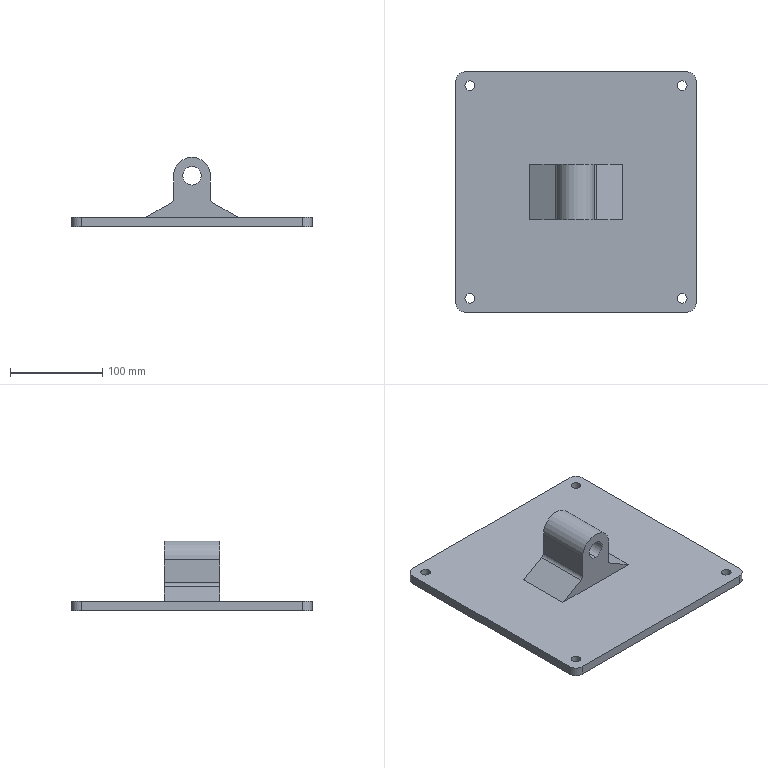Part | SolidWorks | features ICE 2, Extrusion 1, Fillet 1 | 1 solid | 29 faces | box 260 x 260 x 75 mm | volume 829791 mm3 | cylinder 17 | plane 12 | commonest cylinder face diameters 10.5 x8 20 x6 10 x2 40 x1
STEP:
#1=CARTESIAN_POINT('',(0.,30.,45.));
#2=VERTEX_POINT('',#1);
#3=CARTESIAN_POINT('',(0.,30.,65.));
#4=VERTEX_POINT('',#3);
#5=CARTESIAN_POINT('',(0.,30.,55.));
#6=DIRECTION('',(0.,1.,0.));
#7=DIRECTION('',(0.,0.,1.));
#8=AXIS2_PLACEMENT_3D('',#5,#6,#7);
#9=CIRCLE('',#8,10.);
#10=EDGE_CURVE('',#2,#4,#9,.T.);
#11=ORIENTED_EDGE('',*,*,#10,.T.);
#12=CARTESIAN_POINT('',(0.,-30.,65.));
#13=VERTEX_POINT('',#12);
#14=CARTESIAN_POINT('',(0.,104.,65.));
#15=DIRECTION('',(0.,-1.,0.));
#16=VECTOR('',#15,1000.);
#17=LINE('',#14,#16);
#18=EDGE_CURVE('',#4,#13,#17,.T.);
#19=ORIENTED_EDGE('',*,*,#18,.T.);
#20=CARTESIAN_POINT('',(0.,-30.,45.));
#21=VERTEX_POINT('',#20);
#22=CARTESIAN_POINT('',(0.,-30.,55.));
#23=DIRECTION('',(0.,-1.,0.));
#24=DIRECTION('',(0.,0.,-1.));
#25=AXIS2_PLACEMENT_3D('',#22,#23,#24);
#26=CIRCLE('',#25,10.);
#27=EDGE_CURVE('',#13,#21,#26,.T.);
#28=ORIENTED_EDGE('',*,*,#27,.T.);
#29=CARTESIAN_POINT('',(0.,104.,45.));
#30=DIRECTION('',(0.,-1.,0.));
#31=VECTOR('',#30,1000.);
#32=LINE('',#29,#31);
#33=EDGE_CURVE('',#2,#21,#32,.T.);
#34=ORIENTED_EDGE('',*,*,#33,.F.);
#35=EDGE_LOOP('',(#11,#19,#28,#34));
#36=FACE_OUTER_BOUND('',#35,.T.);
#37=CARTESIAN_POINT('',(0.,104.,55.));
#38=DIRECTION('',(0.,-1.,0.));
#39=DIRECTION('',(0.,0.,-1.));
#40=AXIS2_PLACEMENT_3D('',#37,#38,#39);
#41=CYLINDRICAL_SURFACE('',#40,10.);
#42=ADVANCED_FACE('',(#36),#41,.F.);
#43=CARTESIAN_POINT('',(-120.25,-115.,10.));
#44=VERTEX_POINT('',#43);
#45=CARTESIAN_POINT('',(-109.75,-115.,10.));
#46=VERTEX_POINT('',#45);
#47=CARTESIAN_POINT('',(-115.,-115.,10.));
#48=DIRECTION('',(0.,0.,1.));
#49=DIRECTION('',(1.,0.,0.));
#50=AXIS2_PLACEMENT_3D('',#47,#48,#49);
#51=CIRCLE('',#50,5.25);
#52=EDGE_CURVE('',#44,#46,#51,.T.);
#53=ORIENTED_EDGE('',*,*,#52,.T.);
#54=CARTESIAN_POINT('',(-109.75,-115.,0.));
#55=VERTEX_POINT('',#54);
#56=CARTESIAN_POINT('',(-109.75,-115.,10.));
#57=DIRECTION('',(0.,0.,-1.));
#58=VECTOR('',#57,1000.);
#59=LINE('',#56,#58);
#60=EDGE_CURVE('',#46,#55,#59,.T.);
#61=ORIENTED_EDGE('',*,*,#60,.T.);
#62=CARTESIAN_POINT('',(-120.25,-115.,0.));
#63=VERTEX_POINT('',#62);
#64=CARTESIAN_POINT('',(-115.,-115.,0.));
#65=DIRECTION('',(0.,0.,1.));
#66=DIRECTION('',(1.,0.,0.));
#67=AXIS2_PLACEMENT_3D('',#64,#65,#66);
#68=CIRCLE('',#67,5.25);
#69=EDGE_CURVE('',#63,#55,#68,.T.);
#70=ORIENTED_EDGE('',*,*,#69,.F.);
#71=CARTESIAN_POINT('',(-120.25,-115.,10.));
#72=DIRECTION('',(0.,0.,-1.));
#73=VECTOR('',#72,1000.);
#74=LINE('',#71,#73);
#75=EDGE_CURVE('',#44,#63,#74,.T.);
#76=ORIENTED_EDGE('',*,*,#75,.F.);
#77=EDGE_LOOP('',(#53,#61,#70,#76));
#78=FACE_OUTER_BOUND('',#77,.T.);
#79=CARTESIAN_POINT('',(-115.,-115.,10.));
#80=DIRECTION('',(0.,0.,-1.));
#81=DIRECTION('',(-1.,0.,0.));
#82=AXIS2_PLACEMENT_3D('',#79,#80,#81);
#83=CYLINDRICAL_SURFACE('',#82,5.25);
#84=ADVANCED_FACE('',(#78),#83,.F.);
#85=CARTESIAN_POINT('',(109.75,-115.,10.));
#86=VERTEX_POINT('',#85);
#87=CARTESIAN_POINT('',(120.25,-115.,10.));
#88=VERTEX_POINT('',#87);
#89=CARTESIAN_POINT('',(115.,-115.,10.));
#90=DIRECTION('',(0.,0.,1.));
#91=DIRECTION('',(1.,0.,0.));
#92=AXIS2_PLACEMENT_3D('',#89,#90,#91);
#93=CIRCLE('',#92,5.25);
#94=EDGE_CURVE('',#86,#88,#93,.T.);
#95=ORIENTED_EDGE('',*,*,#94,.T.);
#96=CARTESIAN_POINT('',(120.25,-115.,0.));
#97=VERTEX_POINT('',#96);
#98=CARTESIAN_POINT('',(120.25,-115.,10.));
#99=DIRECTION('',(0.,0.,-1.));
#100=VECTOR('',#99,1000.);
#101=LINE('',#98,#100);
#102=EDGE_CURVE('',#88,#97,#101,.T.);
#103=ORIENTED_EDGE('',*,*,#102,.T.);
#104=CARTESIAN_POINT('',(109.75,-115.,0.));
#105=VERTEX_POINT('',#104);
#106=CARTESIAN_POINT('',(115.,-115.,0.));
#107=DIRECTION('',(0.,0.,1.));
#108=DIRECTION('',(1.,0.,0.));
#109=AXIS2_PLACEMENT_3D('',#106,#107,#108);
#110=CIRCLE('',#109,5.25);
#111=EDGE_CURVE('',#105,#97,#110,.T.);
#112=ORIENTED_EDGE('',*,*,#111,.F.);
#113=CARTESIAN_POINT('',(109.75,-115.,10.));
#114=DIRECTION('',(0.,0.,-1.));
#115=VECTOR('',#114,1000.);
#116=LINE('',#113,#115);
#117=EDGE_CURVE('',#86,#105,#116,.T.);
#118=ORIENTED_EDGE('',*,*,#117,.F.);
#119=EDGE_LOOP('',(#95,#103,#112,#118));
#120=FACE_OUTER_BOUND('',#119,.T.);
#121=CARTESIAN_POINT('',(115.,-115.,10.));
#122=DIRECTION('',(0.,0.,-1.));
#123=DIRECTION('',(-1.,0.,0.));
#124=AXIS2_PLACEMENT_3D('',#121,#122,#123);
#125=CYLINDRICAL_SURFACE('',#124,5.25);
#126=ADVANCED_FACE('',(#120),#125,.F.);
#127=CARTESIAN_POINT('',(109.75,115.,10.));
#128=VERTEX_POINT('',#127);
#129=CARTESIAN_POINT('',(120.25,115.,10.));
#130=VERTEX_POINT('',#129);
#131=CARTESIAN_POINT('',(115.,115.,10.));
#132=DIRECTION('',(0.,0.,1.));
#133=DIRECTION('',(1.,0.,0.));
#134=AXIS2_PLACEMENT_3D('',#131,#132,#133);
#135=CIRCLE('',#134,5.25);
#136=EDGE_CURVE('',#128,#130,#135,.T.);
#137=ORIENTED_EDGE('',*,*,#136,.T.);
#138=CARTESIAN_POINT('',(120.25,115.,0.));
#139=VERTEX_POINT('',#138);
#140=CARTESIAN_POINT('',(120.25,115.,10.));
#141=DIRECTION('',(0.,0.,-1.));
#142=VECTOR('',#141,1000.);
#143=LINE('',#140,#142);
#144=EDGE_CURVE('',#130,#139,#143,.T.);
#145=ORIENTED_EDGE('',*,*,#144,.T.);
#146=CARTESIAN_POINT('',(109.75,115.,0.));
#147=VERTEX_POINT('',#146);
#148=CARTESIAN_POINT('',(115.,115.,0.));
#149=DIRECTION('',(0.,0.,1.));
#150=DIRECTION('',(1.,0.,0.));
#151=AXIS2_PLACEMENT_3D('',#148,#149,#150);
#152=CIRCLE('',#151,5.25);
#153=EDGE_CURVE('',#147,#139,#152,.T.);
#154=ORIENTED_EDGE('',*,*,#153,.F.);
#155=CARTESIAN_POINT('',(109.75,115.,10.));
#156=DIRECTION('',(0.,0.,-1.));
#157=VECTOR('',#156,1000.);
#158=LINE('',#155,#157);
#159=EDGE_CURVE('',#128,#147,#158,.T.);
#160=ORIENTED_EDGE('',*,*,#159,.F.);
#161=EDGE_LOOP('',(#137,#145,#154,#160));
#162=FACE_OUTER_BOUND('',#161,.T.);
#163=CARTESIAN_POINT('',(115.,115.,10.));
#164=DIRECTION('',(0.,0.,-1.));
#165=DIRECTION('',(-1.,0.,0.));
#166=AXIS2_PLACEMENT_3D('',#163,#164,#165);
#167=CYLINDRICAL_SURFACE('',#166,5.25);
#168=ADVANCED_FACE('',(#162),#167,.F.);
#169=CARTESIAN_POINT('',(-120.25,115.,10.));
#170=VERTEX_POINT('',#169);
#171=CARTESIAN_POINT('',(-109.75,115.,10.));
#172=VERTEX_POINT('',#171);
#173=CARTESIAN_POINT('',(-115.,115.,10.));
#174=DIRECTION('',(0.,0.,1.));
#175=DIRECTION('',(1.,0.,0.));
#176=AXIS2_PLACEMENT_3D('',#173,#174,#175);
#177=CIRCLE('',#176,5.25);
#178=EDGE_CURVE('',#170,#172,#177,.T.);
#179=ORIENTED_EDGE('',*,*,#178,.T.);
#180=CARTESIAN_POINT('',(-109.75,115.,0.));
#181=VERTEX_POINT('',#180);
#182=CARTESIAN_POINT('',(-109.75,115.,10.));
#183=DIRECTION('',(0.,0.,-1.));
#184=VECTOR('',#183,1000.);
#185=LINE('',#182,#184);
#186=EDGE_CURVE('',#172,#181,#185,.T.);
#187=ORIENTED_EDGE('',*,*,#186,.T.);
#188=CARTESIAN_POINT('',(-120.25,115.,0.));
#189=VERTEX_POINT('',#188);
#190=CARTESIAN_POINT('',(-115.,115.,0.));
#191=DIRECTION('',(0.,0.,1.));
#192=DIRECTION('',(1.,0.,0.));
#193=AXIS2_PLACEMENT_3D('',#190,#191,#192);
#194=CIRCLE('',#193,5.25);
#195=EDGE_CURVE('',#189,#181,#194,.T.);
#196=ORIENTED_EDGE('',*,*,#195,.F.);
#197=CARTESIAN_POINT('',(-120.25,115.,10.));
#198=DIRECTION('',(0.,0.,-1.));
#199=VECTOR('',#198,1000.);
#200=LINE('',#197,#199);
#201=EDGE_CURVE('',#170,#189,#200,.T.);
#202=ORIENTED_EDGE('',*,*,#201,.F.);
#203=EDGE_LOOP('',(#179,#187,#196,#202));
#204=FACE_OUTER_BOUND('',#203,.T.);
#205=CARTESIAN_POINT('',(-115.,115.,10.));
#206=DIRECTION('',(0.,0.,-1.));
#207=DIRECTION('',(-1.,0.,0.));
#208=AXIS2_PLACEMENT_3D('',#205,#206,#207);
#209=CYLINDRICAL_SURFACE('',#208,5.25);
#210=ADVANCED_FACE('',(#204),#209,.F.);
#211=CARTESIAN_POINT('',(-50.,30.,10.));
#212=VERTEX_POINT('',#211);
#213=CARTESIAN_POINT('',(-50.,-30.,10.));
#214=VERTEX_POINT('',#213);
#215=CARTESIAN_POINT('',(-50.,30.,10.));
#216=DIRECTION('',(0.,-1.,0.));
#217=VECTOR('',#216,1000.);
#218=LINE('',#215,#217);
#219=EDGE_CURVE('',#212,#214,#218,.T.);
#220=ORIENTED_EDGE('',*,*,#219,.F.);
#221=CARTESIAN_POINT('',(50.,30.,10.));
#222=VERTEX_POINT('',#221);
#223=CARTESIAN_POINT('',(-50.,30.,10.));
#224=DIRECTION('',(-1.,0.,0.));
#225=VECTOR('',#224,1000.);
#226=LINE('',#223,#225);
#227=EDGE_CURVE('',#222,#212,#226,.T.);
#228=ORIENTED_EDGE('',*,*,#227,.F.);
#229=CARTESIAN_POINT('',(50.,-30.,10.));
#230=VERTEX_POINT('',#229);
#231=CARTESIAN_POINT('',(50.,30.,10.));
#232=DIRECTION('',(0.,-1.,0.));
#233=VECTOR('',#232,1000.);
#234=LINE('',#231,#233);
#235=EDGE_CURVE('',#222,#230,#234,.T.);
#236=ORIENTED_EDGE('',*,*,#235,.T.);
#237=CARTESIAN_POINT('',(-50.,-30.,10.));
#238=DIRECTION('',(-1.,0.,0.));
#239=VECTOR('',#238,1000.);
#240=LINE('',#237,#239);
#241=EDGE_CURVE('',#230,#214,#240,.T.);
#242=ORIENTED_EDGE('',*,*,#241,.T.);
#243=EDGE_LOOP('',(#220,#228,#236,#242));
#244=FACE_BOUND('',#243,.T.);
#245=CARTESIAN_POINT('',(-130.,-120.,10.));
#246=VERTEX_POINT('',#245);
#247=CARTESIAN_POINT('',(-120.,-130.,10.));
#248=VERTEX_POINT('',#247);
#249=CARTESIAN_POINT('',(-120.,-120.,10.));
#250=DIRECTION('',(0.,0.,1.));
#251=DIRECTION('',(-1.,0.,0.));
#252=AXIS2_PLACEMENT_3D('',#249,#250,#251);
#253=CIRCLE('',#252,10.);
#254=EDGE_CURVE('',#246,#248,#253,.T.);
#255=ORIENTED_EDGE('',*,*,#254,.T.);
#256=CARTESIAN_POINT('',(120.,-130.,10.));
#257=VERTEX_POINT('',#256);
#258=CARTESIAN_POINT('',(-120.,-130.,10.));
#259=DIRECTION('',(1.,0.,0.));
#260=VECTOR('',#259,1000.);
#261=LINE('',#258,#260);
#262=EDGE_CURVE('',#248,#257,#261,.T.);
#263=ORIENTED_EDGE('',*,*,#262,.T.);
#264=CARTESIAN_POINT('',(130.,-120.,10.));
#265=VERTEX_POINT('',#264);
#266=CARTESIAN_POINT('',(120.,-120.,10.));
#267=DIRECTION('',(0.,0.,1.));
#268=DIRECTION('',(1.,0.,0.));
#269=AXIS2_PLACEMENT_3D('',#266,#267,#268);
#270=CIRCLE('',#269,10.);
#271=EDGE_CURVE('',#257,#265,#270,.T.);
#272=ORIENTED_EDGE('',*,*,#271,.T.);
#273=CARTESIAN_POINT('',(130.,120.,10.));
#274=VERTEX_POINT('',#273);
#275=CARTESIAN_POINT('',(130.,-120.,10.));
#276=DIRECTION('',(0.,1.,0.));
#277=VECTOR('',#276,1000.);
#278=LINE('',#275,#277);
#279=EDGE_CURVE('',#265,#274,#278,.T.);
#280=ORIENTED_EDGE('',*,*,#279,.T.);
#281=CARTESIAN_POINT('',(120.,130.,10.));
#282=VERTEX_POINT('',#281);
#283=CARTESIAN_POINT('',(120.,120.,10.));
#284=DIRECTION('',(0.,0.,1.));
#285=DIRECTION('',(-1.,0.,0.));
#286=AXIS2_PLACEMENT_3D('',#283,#284,#285);
#287=CIRCLE('',#286,10.);
#288=EDGE_CURVE('',#274,#282,#287,.T.);
#289=ORIENTED_EDGE('',*,*,#288,.T.);
#290=CARTESIAN_POINT('',(-120.,130.,10.));
#291=VERTEX_POINT('',#290);
#292=CARTESIAN_POINT('',(-120.,130.,10.));
#293=DIRECTION('',(-1.,0.,0.));
#294=VECTOR('',#293,1000.);
#295=LINE('',#292,#294);
#296=EDGE_CURVE('',#282,#291,#295,.T.);
#297=ORIENTED_EDGE('',*,*,#296,.T.);
#298=CARTESIAN_POINT('',(-130.,120.,10.));
#299=VERTEX_POINT('',#298);
#300=CARTESIAN_POINT('',(-120.,120.,10.));
#301=DIRECTION('',(0.,0.,1.));
#302=DIRECTION('',(-1.,0.,0.));
#303=AXIS2_PLACEMENT_3D('',#300,#301,#302);
#304=CIRCLE('',#303,10.);
#305=EDGE_CURVE('',#291,#299,#304,.T.);
#306=ORIENTED_EDGE('',*,*,#305,.T.);
#307=CARTESIAN_POINT('',(-130.,-120.,10.));
#308=DIRECTION('',(0.,-1.,0.));
#309=VECTOR('',#308,1000.);
#310=LINE('',#307,#309);
#311=EDGE_CURVE('',#299,#246,#310,.T.);
#312=ORIENTED_EDGE('',*,*,#311,.T.);
#313=EDGE_LOOP('',(#255,#263,#272,#280,#289,#297,#306,#312));
#314=FACE_OUTER_BOUND('',#313,.T.);
#315=ORIENTED_EDGE('',*,*,#178,.F.);
#316=CARTESIAN_POINT('',(-115.,115.,10.));
#317=DIRECTION('',(0.,0.,1.));
#318=DIRECTION('',(1.,0.,0.));
#319=AXIS2_PLACEMENT_3D('',#316,#317,#318);
#320=CIRCLE('',#319,5.25);
#321=EDGE_CURVE('',#172,#170,#320,.T.);
#322=ORIENTED_EDGE('',*,*,#321,.F.);
#323=EDGE_LOOP('',(#315,#322));
#324=FACE_BOUND('',#323,.T.);
#325=ORIENTED_EDGE('',*,*,#136,.F.);
#326=CARTESIAN_POINT('',(115.,115.,10.));
#327=DIRECTION('',(0.,0.,1.));
#328=DIRECTION('',(1.,0.,0.));
#329=AXIS2_PLACEMENT_3D('',#326,#327,#328);
#330=CIRCLE('',#329,5.25);
#331=EDGE_CURVE('',#130,#128,#330,.T.);
#332=ORIENTED_EDGE('',*,*,#331,.F.);
#333=EDGE_LOOP('',(#325,#332));
#334=FACE_BOUND('',#333,.T.);
#335=ORIENTED_EDGE('',*,*,#94,.F.);
#336=CARTESIAN_POINT('',(115.,-115.,10.));
#337=DIRECTION('',(0.,0.,1.));
#338=DIRECTION('',(1.,0.,0.));
#339=AXIS2_PLACEMENT_3D('',#336,#337,#338);
#340=CIRCLE('',#339,5.25);
#341=EDGE_CURVE('',#88,#86,#340,.T.);
#342=ORIENTED_EDGE('',*,*,#341,.F.);
#343=EDGE_LOOP('',(#335,#342));
#344=FACE_BOUND('',#343,.T.);
#345=ORIENTED_EDGE('',*,*,#52,.F.);
#346=CARTESIAN_POINT('',(-115.,-115.,10.));
#347=DIRECTION('',(0.,0.,1.));
#348=DIRECTION('',(1.,0.,0.));
#349=AXIS2_PLACEMENT_3D('',#346,#347,#348);
#350=CIRCLE('',#349,5.25);
#351=EDGE_CURVE('',#46,#44,#350,.T.);
#352=ORIENTED_EDGE('',*,*,#351,.F.);
#353=EDGE_LOOP('',(#345,#352));
#354=FACE_BOUND('',#353,.T.);
#355=CARTESIAN_POINT('',(-120.,-120.,10.));
#356=DIRECTION('',(0.,0.,-1.));
#357=DIRECTION('',(-1.,0.,0.));
#358=AXIS2_PLACEMENT_3D('',#355,#356,#357);
#359=PLANE('',#358);
#360=ADVANCED_FACE('',(#244,#314,#324,#334,#344,#354),#359,.F.);
#361=ORIENTED_EDGE('',*,*,#111,.T.);
#362=CARTESIAN_POINT('',(115.,-115.,0.));
#363=DIRECTION('',(0.,0.,1.));
#364=DIRECTION('',(1.,0.,0.));
#365=AXIS2_PLACEMENT_3D('',#362,#363,#364);
#366=CIRCLE('',#365,5.25);
#367=EDGE_CURVE('',#97,#105,#366,.T.);
#368=ORIENTED_EDGE('',*,*,#367,.T.);
#369=EDGE_LOOP('',(#361,#368));
#370=FACE_BOUND('',#369,.T.);
#371=ORIENTED_EDGE('',*,*,#195,.T.);
#372=CARTESIAN_POINT('',(-115.,115.,0.));
#373=DIRECTION('',(0.,0.,1.));
#374=DIRECTION('',(1.,0.,0.));
#375=AXIS2_PLACEMENT_3D('',#372,#373,#374);
#376=CIRCLE('',#375,5.25);
#377=EDGE_CURVE('',#181,#189,#376,.T.);
#378=ORIENTED_EDGE('',*,*,#377,.T.);
#379=EDGE_LOOP('',(#371,#378));
#380=FACE_BOUND('',#379,.T.);
#381=CARTESIAN_POINT('',(-130.,-120.,0.));
#382=VERTEX_POINT('',#381);
#383=CARTESIAN_POINT('',(-120.,-130.,0.));
#384=VERTEX_POINT('',#383);
#385=CARTESIAN_POINT('',(-120.,-120.,0.));
#386=DIRECTION('',(0.,0.,1.));
#387=DIRECTION('',(-1.,0.,0.));
#388=AXIS2_PLACEMENT_3D('',#385,#386,#387);
#389=CIRCLE('',#388,10.);
#390=EDGE_CURVE('',#382,#384,#389,.T.);
#391=ORIENTED_EDGE('',*,*,#390,.F.);
#392=CARTESIAN_POINT('',(-130.,120.,0.));
#393=VERTEX_POINT('',#392);
#394=CARTESIAN_POINT('',(-130.,-120.,0.));
#395=DIRECTION('',(0.,-1.,0.));
#396=VECTOR('',#395,1000.);
#397=LINE('',#394,#396);
#398=EDGE_CURVE('',#393,#382,#397,.T.);
#399=ORIENTED_EDGE('',*,*,#398,.F.);
#400=CARTESIAN_POINT('',(-120.,130.,0.));
#401=VERTEX_POINT('',#400);
#402=CARTESIAN_POINT('',(-120.,120.,0.));
#403=DIRECTION('',(0.,0.,1.));
#404=DIRECTION('',(-1.,0.,0.));
#405=AXIS2_PLACEMENT_3D('',#402,#403,#404);
#406=CIRCLE('',#405,10.);
#407=EDGE_CURVE('',#401,#393,#406,.T.);
#408=ORIENTED_EDGE('',*,*,#407,.F.);
#409=CARTESIAN_POINT('',(120.,130.,0.));
#410=VERTEX_POINT('',#409);
#411=CARTESIAN_POINT('',(-120.,130.,0.));
#412=DIRECTION('',(-1.,0.,0.));
#413=VECTOR('',#412,1000.);
#414=LINE('',#411,#413);
#415=EDGE_CURVE('',#410,#401,#414,.T.);
#416=ORIENTED_EDGE('',*,*,#415,.F.);
#417=CARTESIAN_POINT('',(130.,120.,0.));
#418=VERTEX_POINT('',#417);
#419=CARTESIAN_POINT('',(120.,120.,0.));
#420=DIRECTION('',(0.,0.,1.));
#421=DIRECTION('',(-1.,0.,0.));
#422=AXIS2_PLACEMENT_3D('',#419,#420,#421);
#423=CIRCLE('',#422,10.);
#424=EDGE_CURVE('',#418,#410,#423,.T.);
#425=ORIENTED_EDGE('',*,*,#424,.F.);
#426=CARTESIAN_POINT('',(130.,-120.,0.));
#427=VERTEX_POINT('',#426);
#428=CARTESIAN_POINT('',(130.,-120.,0.));
#429=DIRECTION('',(0.,1.,0.));
#430=VECTOR('',#429,1000.);
#431=LINE('',#428,#430);
#432=EDGE_CURVE('',#427,#418,#431,.T.);
#433=ORIENTED_EDGE('',*,*,#432,.F.);
#434=CARTESIAN_POINT('',(120.,-130.,0.));
#435=VERTEX_POINT('',#434);
#436=CARTESIAN_POINT('',(120.,-120.,0.));
#437=DIRECTION('',(0.,0.,1.));
#438=DIRECTION('',(1.,0.,0.));
#439=AXIS2_PLACEMENT_3D('',#436,#437,#438);
#440=CIRCLE('',#439,10.);
#441=EDGE_CURVE('',#435,#427,#440,.T.);
#442=ORIENTED_EDGE('',*,*,#441,.F.);
#443=CARTESIAN_POINT('',(-120.,-130.,0.));
#444=DIRECTION('',(1.,0.,0.));
#445=VECTOR('',#444,1000.);
#446=LINE('',#443,#445);
#447=EDGE_CURVE('',#384,#435,#446,.T.);
#448=ORIENTED_EDGE('',*,*,#447,.F.);
#449=EDGE_LOOP('',(#391,#399,#408,#416,#425,#433,#442,#448));
#450=FACE_OUTER_BOUND('',#449,.T.);
#451=ORIENTED_EDGE('',*,*,#153,.T.);
#452=CARTESIAN_POINT('',(115.,115.,0.));
#453=DIRECTION('',(0.,0.,1.));
#454=DIRECTION('',(1.,0.,0.));
#455=AXIS2_PLACEMENT_3D('',#452,#453,#454);
#456=CIRCLE('',#455,5.25);
#457=EDGE_CURVE('',#139,#147,#456,.T.);
#458=ORIENTED_EDGE('',*,*,#457,.T.);
#459=EDGE_LOOP('',(#451,#458));
#460=FACE_BOUND('',#459,.T.);
#461=ORIENTED_EDGE('',*,*,#69,.T.);
#462=CARTESIAN_POINT('',(-115.,-115.,0.));
#463=DIRECTION('',(0.,0.,1.));
#464=DIRECTION('',(1.,0.,0.));
#465=AXIS2_PLACEMENT_3D('',#462,#463,#464);
#466=CIRCLE('',#465,5.25);
#467=EDGE_CURVE('',#55,#63,#466,.T.);
#468=ORIENTED_EDGE('',*,*,#467,.T.);
#469=EDGE_LOOP('',(#461,#468));
#470=FACE_BOUND('',#469,.T.);
#471=CARTESIAN_POINT('',(-120.,-120.,0.));
#472=DIRECTION('',(0.,0.,-1.));
#473=DIRECTION('',(-1.,0.,0.));
#474=AXIS2_PLACEMENT_3D('',#471,#472,#473);
#475=PLANE('',#474);
#476=ADVANCED_FACE('',(#370,#380,#450,#460,#470),#475,.T.);
#477=ORIENTED_EDGE('',*,*,#390,.T.);
#478=CARTESIAN_POINT('',(-120.,-130.,10.));
#479=DIRECTION('',(0.,0.,-1.));
#480=VECTOR('',#479,1000.);
#481=LINE('',#478,#480);
#482=EDGE_CURVE('',#248,#384,#481,.T.);
#483=ORIENTED_EDGE('',*,*,#482,.F.);
#484=ORIENTED_EDGE('',*,*,#254,.F.);
#485=CARTESIAN_POINT('',(-130.,-120.,10.));
#486=DIRECTION('',(0.,0.,-1.));
#487=VECTOR('',#486,1000.);
#488=LINE('',#485,#487);
#489=EDGE_CURVE('',#246,#382,#488,.T.);
#490=ORIENTED_EDGE('',*,*,#489,.T.);
#491=EDGE_LOOP('',(#477,#483,#484,#490));
#492=FACE_OUTER_BOUND('',#491,.T.);
#493=CARTESIAN_POINT('',(-120.,-120.,10.));
#494=DIRECTION('',(0.,0.,-1.));
#495=DIRECTION('',(-1.,0.,0.));
#496=AXIS2_PLACEMENT_3D('',#493,#494,#495);
#497=CYLINDRICAL_SURFACE('',#496,10.);
#498=ADVANCED_FACE('',(#492),#497,.T.);
#499=ORIENTED_EDGE('',*,*,#447,.T.);
#500=CARTESIAN_POINT('',(120.,-130.,10.));
#501=DIRECTION('',(0.,0.,-1.));
#502=VECTOR('',#501,1000.);
#503=LINE('',#500,#502);
#504=EDGE_CURVE('',#257,#435,#503,.T.);
#505=ORIENTED_EDGE('',*,*,#504,.F.);
#506=ORIENTED_EDGE('',*,*,#262,.F.);
#507=ORIENTED_EDGE('',*,*,#482,.T.);
#508=EDGE_LOOP('',(#499,#505,#506,#507));
#509=FACE_OUTER_BOUND('',#508,.T.);
#510=CARTESIAN_POINT('',(-120.,-130.,10.));
#511=DIRECTION('',(0.,1.,0.));
#512=DIRECTION('',(0.,0.,1.));
#513=AXIS2_PLACEMENT_3D('',#510,#511,#512);
#514=PLANE('',#513);
#515=ADVANCED_FACE('',(#509),#514,.F.);
#516=ORIENTED_EDGE('',*,*,#441,.T.);
#517=CARTESIAN_POINT('',(130.,-120.,10.));
#518=DIRECTION('',(0.,0.,-1.));
#519=VECTOR('',#518,1000.);
#520=LINE('',#517,#519);
#521=EDGE_CURVE('',#265,#427,#520,.T.);
#522=ORIENTED_EDGE('',*,*,#521,.F.);
#523=ORIENTED_EDGE('',*,*,#271,.F.);
#524=ORIENTED_EDGE('',*,*,#504,.T.);
#525=EDGE_LOOP('',(#516,#522,#523,#524));
#526=FACE_OUTER_BOUND('',#525,.T.);
#527=CARTESIAN_POINT('',(120.,-120.,10.));
#528=DIRECTION('',(0.,0.,-1.));
#529=DIRECTION('',(-1.,0.,0.));
#530=AXIS2_PLACEMENT_3D('',#527,#528,#529);
#531=CYLINDRICAL_SURFACE('',#530,10.);
#532=ADVANCED_FACE('',(#526),#531,.T.);
#533=ORIENTED_EDGE('',*,*,#432,.T.);
#534=CARTESIAN_POINT('',(130.,120.,10.));
#535=DIRECTION('',(0.,0.,-1.));
#536=VECTOR('',#535,1000.);
#537=LINE('',#534,#536);
#538=EDGE_CURVE('',#274,#418,#537,.T.);
#539=ORIENTED_EDGE('',*,*,#538,.F.);
#540=ORIENTED_EDGE('',*,*,#279,.F.);
#541=ORIENTED_EDGE('',*,*,#521,.T.);
#542=EDGE_LOOP('',(#533,#539,#540,#541));
#543=FACE_OUTER_BOUND('',#542,.T.);
#544=CARTESIAN_POINT('',(130.,-120.,10.));
#545=DIRECTION('',(-1.,0.,0.));
#546=DIRECTION('',(0.,-1.,0.));
#547=AXIS2_PLACEMENT_3D('',#544,#545,#546);
#548=PLANE('',#547);
#549=ADVANCED_FACE('',(#543),#548,.F.);
#550=ORIENTED_EDGE('',*,*,#424,.T.);
#551=CARTESIAN_POINT('',(120.,130.,10.));
#552=DIRECTION('',(0.,0.,-1.));
#553=VECTOR('',#552,1000.);
#554=LINE('',#551,#553);
#555=EDGE_CURVE('',#282,#410,#554,.T.);
#556=ORIENTED_EDGE('',*,*,#555,.F.);
#557=ORIENTED_EDGE('',*,*,#288,.F.);
#558=ORIENTED_EDGE('',*,*,#538,.T.);
#559=EDGE_LOOP('',(#550,#556,#557,#558));
#560=FACE_OUTER_BOUND('',#559,.T.);
#561=CARTESIAN_POINT('',(120.,120.,10.));
#562=DIRECTION('',(0.,0.,-1.));
#563=DIRECTION('',(-1.,0.,0.));
#564=AXIS2_PLACEMENT_3D('',#561,#562,#563);
#565=CYLINDRICAL_SURFACE('',#564,10.);
#566=ADVANCED_FACE('',(#560),#565,.T.);
#567=ORIENTED_EDGE('',*,*,#415,.T.);
#568=CARTESIAN_POINT('',(-120.,130.,10.));
#569=DIRECTION('',(0.,0.,-1.));
#570=VECTOR('',#569,1000.);
#571=LINE('',#568,#570);
#572=EDGE_CURVE('',#291,#401,#571,.T.);
#573=ORIENTED_EDGE('',*,*,#572,.F.);
#574=ORIENTED_EDGE('',*,*,#296,.F.);
#575=ORIENTED_EDGE('',*,*,#555,.T.);
#576=EDGE_LOOP('',(#567,#573,#574,#575));
#577=FACE_OUTER_BOUND('',#576,.T.);
#578=CARTESIAN_POINT('',(-120.,130.,10.));
#579=DIRECTION('',(0.,-1.,0.));
#580=DIRECTION('',(0.,0.,-1.));
#581=AXIS2_PLACEMENT_3D('',#578,#579,#580);
#582=PLANE('',#581);
#583=ADVANCED_FACE('',(#577),#582,.F.);
#584=ORIENTED_EDGE('',*,*,#407,.T.);
#585=CARTESIAN_POINT('',(-130.,120.,10.));
#586=DIRECTION('',(0.,0.,-1.));
#587=VECTOR('',#586,1000.);
#588=LINE('',#585,#587);
#589=EDGE_CURVE('',#299,#393,#588,.T.);
#590=ORIENTED_EDGE('',*,*,#589,.F.);
#591=ORIENTED_EDGE('',*,*,#305,.F.);
#592=ORIENTED_EDGE('',*,*,#572,.T.);
#593=EDGE_LOOP('',(#584,#590,#591,#592));
#594=FACE_OUTER_BOUND('',#593,.T.);
#595=CARTESIAN_POINT('',(-120.,120.,10.));
#596=DIRECTION('',(0.,0.,-1.));
#597=DIRECTION('',(-1.,0.,0.));
#598=AXIS2_PLACEMENT_3D('',#595,#596,#597);
#599=CYLINDRICAL_SURFACE('',#598,10.);
#600=ADVANCED_FACE('',(#594),#599,.T.);
#601=ORIENTED_EDGE('',*,*,#398,.T.);
#602=ORIENTED_EDGE('',*,*,#489,.F.);
#603=ORIENTED_EDGE('',*,*,#311,.F.);
#604=ORIENTED_EDGE('',*,*,#589,.T.);
#605=EDGE_LOOP('',(#601,#602,#603,#604));
#606=FACE_OUTER_BOUND('',#605,.T.);
#607=CARTESIAN_POINT('',(-130.,-120.,10.));
#608=DIRECTION('',(1.,0.,0.));
#609=DIRECTION('',(0.,0.,-1.));
#610=AXIS2_PLACEMENT_3D('',#607,#608,#609);
#611=PLANE('',#610);
#612=ADVANCED_FACE('',(#606),#611,.F.);
#613=ORIENTED_EDGE('',*,*,#186,.F.);
#614=ORIENTED_EDGE('',*,*,#321,.T.);
#615=ORIENTED_EDGE('',*,*,#201,.T.);
#616=ORIENTED_EDGE('',*,*,#377,.F.);
#617=EDGE_LOOP('',(#613,#614,#615,#616));
#618=FACE_OUTER_BOUND('',#617,.T.);
#619=CARTESIAN_POINT('',(-115.,115.,10.));
#620=DIRECTION('',(0.,0.,-1.));
#621=DIRECTION('',(-1.,0.,0.));
#622=AXIS2_PLACEMENT_3D('',#619,#620,#621);
#623=CYLINDRICAL_SURFACE('',#622,5.25);
#624=ADVANCED_FACE('',(#618),#623,.F.);
#625=ORIENTED_EDGE('',*,*,#144,.F.);
#626=ORIENTED_EDGE('',*,*,#331,.T.);
#627=ORIENTED_EDGE('',*,*,#159,.T.);
#628=ORIENTED_EDGE('',*,*,#457,.F.);
#629=EDGE_LOOP('',(#625,#626,#627,#628));
#630=FACE_OUTER_BOUND('',#629,.T.);
#631=CARTESIAN_POINT('',(115.,115.,10.));
#632=DIRECTION('',(0.,0.,-1.));
#633=DIRECTION('',(-1.,0.,0.));
#634=AXIS2_PLACEMENT_3D('',#631,#632,#633);
#635=CYLINDRICAL_SURFACE('',#634,5.25);
#636=ADVANCED_FACE('',(#630),#635,.F.);
#637=ORIENTED_EDGE('',*,*,#102,.F.);
#638=ORIENTED_EDGE('',*,*,#341,.T.);
#639=ORIENTED_EDGE('',*,*,#117,.T.);
#640=ORIENTED_EDGE('',*,*,#367,.F.);
#641=EDGE_LOOP('',(#637,#638,#639,#640));
#642=FACE_OUTER_BOUND('',#641,.T.);
#643=CARTESIAN_POINT('',(115.,-115.,10.));
#644=DIRECTION('',(0.,0.,-1.));
#645=DIRECTION('',(-1.,0.,0.));
#646=AXIS2_PLACEMENT_3D('',#643,#644,#645);
#647=CYLINDRICAL_SURFACE('',#646,5.25);
#648=ADVANCED_FACE('',(#642),#647,.F.);
#649=ORIENTED_EDGE('',*,*,#60,.F.);
#650=ORIENTED_EDGE('',*,*,#351,.T.);
#651=ORIENTED_EDGE('',*,*,#75,.T.);
#652=ORIENTED_EDGE('',*,*,#467,.F.);
#653=EDGE_LOOP('',(#649,#650,#651,#652));
#654=FACE_OUTER_BOUND('',#653,.T.);
#655=CARTESIAN_POINT('',(-115.,-115.,10.));
#656=DIRECTION('',(0.,0.,-1.));
#657=DIRECTION('',(-1.,0.,0.));
#658=AXIS2_PLACEMENT_3D('',#655,#656,#657);
#659=CYLINDRICAL_SURFACE('',#658,5.25);
#660=ADVANCED_FACE('',(#654),#659,.F.);
#661=CARTESIAN_POINT('',(-22.505,-30.,25.836));
#662=VERTEX_POINT('',#661);
#663=CARTESIAN_POINT('',(-50.,-30.,10.));
#664=DIRECTION('',(0.8665,0.,0.4991));
#665=VECTOR('',#664,1000.);
#666=LINE('',#663,#665);
#667=EDGE_CURVE('',#214,#662,#666,.T.);
#668=ORIENTED_EDGE('',*,*,#667,.T.);
#669=CARTESIAN_POINT('',(-22.505,30.,25.836));
#670=VERTEX_POINT('',#669);
#671=CARTESIAN_POINT('',(-22.505,30.,25.836));
#672=DIRECTION('',(0.,1.,0.));
#673=VECTOR('',#672,1000.);
#674=LINE('',#671,#673);
#675=EDGE_CURVE('',#662,#670,#674,.T.);
#676=ORIENTED_EDGE('',*,*,#675,.T.);
#677=CARTESIAN_POINT('',(-50.,30.,10.));
#678=DIRECTION('',(0.8665,0.,0.4991));
#679=VECTOR('',#678,1000.);
#680=LINE('',#677,#679);
#681=EDGE_CURVE('',#212,#670,#680,.T.);
#682=ORIENTED_EDGE('',*,*,#681,.F.);
#683=ORIENTED_EDGE('',*,*,#219,.T.);
#684=EDGE_LOOP('',(#668,#676,#682,#683));
#685=FACE_OUTER_BOUND('',#684,.T.);
#686=CARTESIAN_POINT('',(-50.,30.,10.));
#687=DIRECTION('',(0.4991,0.,-0.8665));
#688=DIRECTION('',(-0.8665,0.,-0.4991));
#689=AXIS2_PLACEMENT_3D('',#686,#687,#688);
#690=PLANE('',#689);
#691=ADVANCED_FACE('',(#685),#690,.F.);
#692=CARTESIAN_POINT('',(-20.,30.,30.169));
#693=VERTEX_POINT('',#692);
#694=CARTESIAN_POINT('',(-20.,30.,55.));
#695=VERTEX_POINT('',#694);
#696=CARTESIAN_POINT('',(-20.,30.,27.279));
#697=DIRECTION('',(0.,0.,1.));
#698=VECTOR('',#697,1000.);
#699=LINE('',#696,#698);
#700=EDGE_CURVE('',#693,#695,#699,.T.);
#701=ORIENTED_EDGE('',*,*,#700,.F.);
#702=CARTESIAN_POINT('',(-20.,-30.,30.169));
#703=VERTEX_POINT('',#702);
#704=CARTESIAN_POINT('',(-20.,-30.,30.169));
#705=DIRECTION('',(0.,-1.,0.));
#706=VECTOR('',#705,1000.);
#707=LINE('',#704,#706);
#708=EDGE_CURVE('',#693,#703,#707,.T.);
#709=ORIENTED_EDGE('',*,*,#708,.T.);
#710=CARTESIAN_POINT('',(-20.,-30.,55.));
#711=VERTEX_POINT('',#710);
#712=CARTESIAN_POINT('',(-20.,-30.,27.279));
#713=DIRECTION('',(0.,0.,1.));
#714=VECTOR('',#713,1000.);
#715=LINE('',#712,#714);
#716=EDGE_CURVE('',#703,#711,#715,.T.);
#717=ORIENTED_EDGE('',*,*,#716,.T.);
#718=CARTESIAN_POINT('',(-20.,30.,55.));
#719=DIRECTION('',(0.,-1.,0.));
#720=VECTOR('',#719,1000.);
#721=LINE('',#718,#720);
#722=EDGE_CURVE('',#695,#711,#721,.T.);
#723=ORIENTED_EDGE('',*,*,#722,.F.);
#724=EDGE_LOOP('',(#701,#709,#717,#723));
#725=FACE_OUTER_BOUND('',#724,.T.);
#726=CARTESIAN_POINT('',(-20.,30.,27.279));
#727=DIRECTION('',(1.,0.,0.));
#728=DIRECTION('',(0.,0.,-1.));
#729=AXIS2_PLACEMENT_3D('',#726,#727,#728);
#730=PLANE('',#729);
#731=ADVANCED_FACE('',(#725),#730,.F.);
#732=CARTESIAN_POINT('',(20.,-30.,55.));
#733=VERTEX_POINT('',#732);
#734=CARTESIAN_POINT('',(0.,-30.,55.));
#735=DIRECTION('',(0.,1.,0.));
#736=DIRECTION('',(0.,0.,1.));
#737=AXIS2_PLACEMENT_3D('',#734,#735,#736);
#738=CIRCLE('',#737,20.);
#739=EDGE_CURVE('',#711,#733,#738,.T.);
#740=ORIENTED_EDGE('',*,*,#739,.T.);
#741=CARTESIAN_POINT('',(20.,30.,55.));
#742=VERTEX_POINT('',#741);
#743=CARTESIAN_POINT('',(20.,30.,55.));
#744=DIRECTION('',(0.,-1.,0.));
#745=VECTOR('',#744,1000.);
#746=LINE('',#743,#745);
#747=EDGE_CURVE('',#742,#733,#746,.T.);
#748=ORIENTED_EDGE('',*,*,#747,.F.);
#749=CARTESIAN_POINT('',(0.,30.,55.));
#750=DIRECTION('',(0.,1.,0.));
#751=DIRECTION('',(0.,0.,1.));
#752=AXIS2_PLACEMENT_3D('',#749,#750,#751);
#753=CIRCLE('',#752,20.);
#754=EDGE_CURVE('',#695,#742,#753,.T.);
#755=ORIENTED_EDGE('',*,*,#754,.F.);
#756=ORIENTED_EDGE('',*,*,#722,.T.);
#757=EDGE_LOOP('',(#740,#748,#755,#756));
#758=FACE_OUTER_BOUND('',#757,.T.);
#759=CARTESIAN_POINT('',(0.,30.,55.));
#760=DIRECTION('',(0.,-1.,0.));
#761=DIRECTION('',(0.,0.,-1.));
#762=AXIS2_PLACEMENT_3D('',#759,#760,#761);
#763=CYLINDRICAL_SURFACE('',#762,20.);
#764=ADVANCED_FACE('',(#758),#763,.T.);
#765=CARTESIAN_POINT('',(20.,-30.,30.169));
#766=VERTEX_POINT('',#765);
#767=CARTESIAN_POINT('',(20.,-30.,55.));
#768=DIRECTION('',(0.,0.,-1.));
#769=VECTOR('',#768,1000.);
#770=LINE('',#767,#769);
#771=EDGE_CURVE('',#733,#766,#770,.T.);
#772=ORIENTED_EDGE('',*,*,#771,.T.);
#773=CARTESIAN_POINT('',(20.,30.,30.169));
#774=VERTEX_POINT('',#773);
#775=CARTESIAN_POINT('',(20.,30.,30.169));
#776=DIRECTION('',(0.,1.,0.));
#777=VECTOR('',#776,1000.);
#778=LINE('',#775,#777);
#779=EDGE_CURVE('',#766,#774,#778,.T.);
#780=ORIENTED_EDGE('',*,*,#779,.T.);
#781=CARTESIAN_POINT('',(20.,30.,55.));
#782=DIRECTION('',(0.,0.,-1.));
#783=VECTOR('',#782,1000.);
#784=LINE('',#781,#783);
#785=EDGE_CURVE('',#742,#774,#784,.T.);
#786=ORIENTED_EDGE('',*,*,#785,.F.);
#787=ORIENTED_EDGE('',*,*,#747,.T.);
#788=EDGE_LOOP('',(#772,#780,#786,#787));
#789=FACE_OUTER_BOUND('',#788,.T.);
#790=CARTESIAN_POINT('',(20.,30.,55.));
#791=DIRECTION('',(-1.,0.,0.));
#792=DIRECTION('',(0.,0.,1.));
#793=AXIS2_PLACEMENT_3D('',#790,#791,#792);
#794=PLANE('',#793);
#795=ADVANCED_FACE('',(#789),#794,.F.);
#796=CARTESIAN_POINT('',(22.505,30.,25.836));
#797=VERTEX_POINT('',#796);
#798=CARTESIAN_POINT('',(20.,30.,27.279));
#799=DIRECTION('',(0.8665,0.,-0.4991));
#800=VECTOR('',#799,1000.);
#801=LINE('',#798,#800);
#802=EDGE_CURVE('',#797,#222,#801,.T.);
#803=ORIENTED_EDGE('',*,*,#802,.F.);
#804=CARTESIAN_POINT('',(22.505,-30.,25.836));
#805=VERTEX_POINT('',#804);
#806=CARTESIAN_POINT('',(22.505,-30.,25.836));
#807=DIRECTION('',(0.,-1.,0.));
#808=VECTOR('',#807,1000.);
#809=LINE('',#806,#808);
#810=EDGE_CURVE('',#797,#805,#809,.T.);
#811=ORIENTED_EDGE('',*,*,#810,.T.);
#812=CARTESIAN_POINT('',(20.,-30.,27.279));
#813=DIRECTION('',(0.8665,0.,-0.4991));
#814=VECTOR('',#813,1000.);
#815=LINE('',#812,#814);
#816=EDGE_CURVE('',#805,#230,#815,.T.);
#817=ORIENTED_EDGE('',*,*,#816,.T.);
#818=ORIENTED_EDGE('',*,*,#235,.F.);
#819=EDGE_LOOP('',(#803,#811,#817,#818));
#820=FACE_OUTER_BOUND('',#819,.T.);
#821=CARTESIAN_POINT('',(20.,30.,27.279));
#822=DIRECTION('',(-0.4991,0.,-0.8665));
#823=DIRECTION('',(-0.8665,0.,0.4991));
#824=AXIS2_PLACEMENT_3D('',#821,#822,#823);
#825=PLANE('',#824);
#826=ADVANCED_FACE('',(#820),#825,.F.);
#827=ORIENTED_EDGE('',*,*,#10,.F.);
#828=CARTESIAN_POINT('',(0.,30.,55.));
#829=DIRECTION('',(0.,1.,0.));
#830=DIRECTION('',(0.,0.,1.));
#831=AXIS2_PLACEMENT_3D('',#828,#829,#830);
#832=CIRCLE('',#831,10.);
#833=EDGE_CURVE('',#4,#2,#832,.T.);
#834=ORIENTED_EDGE('',*,*,#833,.F.);
#835=EDGE_LOOP('',(#827,#834));
#836=FACE_BOUND('',#835,.T.);
#837=ORIENTED_EDGE('',*,*,#681,.T.);
#838=CARTESIAN_POINT('',(-25.,30.,30.169));
#839=DIRECTION('',(0.,-1.,0.));
#840=DIRECTION('',(0.,0.,1.));
#841=AXIS2_PLACEMENT_3D('',#838,#839,#840);
#842=CIRCLE('',#841,5.);
#843=EDGE_CURVE('',#670,#693,#842,.T.);
#844=ORIENTED_EDGE('',*,*,#843,.T.);
#845=ORIENTED_EDGE('',*,*,#700,.T.);
#846=ORIENTED_EDGE('',*,*,#754,.T.);
#847=ORIENTED_EDGE('',*,*,#785,.T.);
#848=CARTESIAN_POINT('',(25.,30.,30.169));
#849=DIRECTION('',(0.,-1.,0.));
#850=DIRECTION('',(0.,0.,1.));
#851=AXIS2_PLACEMENT_3D('',#848,#849,#850);
#852=CIRCLE('',#851,5.);
#853=EDGE_CURVE('',#774,#797,#852,.T.);
#854=ORIENTED_EDGE('',*,*,#853,.T.);
#855=ORIENTED_EDGE('',*,*,#802,.T.);
#856=ORIENTED_EDGE('',*,*,#227,.T.);
#857=EDGE_LOOP('',(#837,#844,#845,#846,#847,#854,#855,#856));
#858=FACE_OUTER_BOUND('',#857,.T.);
#859=CARTESIAN_POINT('',(0.,30.,55.));
#860=DIRECTION('',(0.,1.,0.));
#861=DIRECTION('',(0.,0.,1.));
#862=AXIS2_PLACEMENT_3D('',#859,#860,#861);
#863=PLANE('',#862);
#864=ADVANCED_FACE('',(#836,#858),#863,.T.);
#865=CARTESIAN_POINT('',(0.,-30.,55.));
#866=DIRECTION('',(0.,-1.,0.));
#867=DIRECTION('',(0.,0.,-1.));
#868=AXIS2_PLACEMENT_3D('',#865,#866,#867);
#869=CIRCLE('',#868,10.);
#870=EDGE_CURVE('',#21,#13,#869,.T.);
#871=ORIENTED_EDGE('',*,*,#870,.F.);
#872=ORIENTED_EDGE('',*,*,#27,.F.);
#873=EDGE_LOOP('',(#871,#872));
#874=FACE_BOUND('',#873,.T.);
#875=ORIENTED_EDGE('',*,*,#667,.F.);
#876=ORIENTED_EDGE('',*,*,#241,.F.);
#877=ORIENTED_EDGE('',*,*,#816,.F.);
#878=CARTESIAN_POINT('',(25.,-30.,30.169));
#879=DIRECTION('',(0.,1.,0.));
#880=DIRECTION('',(0.,0.,1.));
#881=AXIS2_PLACEMENT_3D('',#878,#879,#880);
#882=CIRCLE('',#881,5.);
#883=EDGE_CURVE('',#805,#766,#882,.T.);
#884=ORIENTED_EDGE('',*,*,#883,.T.);
#885=ORIENTED_EDGE('',*,*,#771,.F.);
#886=ORIENTED_EDGE('',*,*,#739,.F.);
#887=ORIENTED_EDGE('',*,*,#716,.F.);
#888=CARTESIAN_POINT('',(-25.,-30.,30.169));
#889=DIRECTION('',(0.,1.,0.));
#890=DIRECTION('',(0.,0.,1.));
#891=AXIS2_PLACEMENT_3D('',#888,#889,#890);
#892=CIRCLE('',#891,5.);
#893=EDGE_CURVE('',#703,#662,#892,.T.);
#894=ORIENTED_EDGE('',*,*,#893,.T.);
#895=EDGE_LOOP('',(#875,#876,#877,#884,#885,#886,#887,#894));
#896=FACE_OUTER_BOUND('',#895,.T.);
#897=CARTESIAN_POINT('',(0.,-30.,55.));
#898=DIRECTION('',(0.,1.,0.));
#899=DIRECTION('',(0.,0.,1.));
#900=AXIS2_PLACEMENT_3D('',#897,#898,#899);
#901=PLANE('',#900);
#902=ADVANCED_FACE('',(#874,#896),#901,.F.);
#903=ORIENTED_EDGE('',*,*,#18,.F.);
#904=ORIENTED_EDGE('',*,*,#833,.T.);
#905=ORIENTED_EDGE('',*,*,#33,.T.);
#906=ORIENTED_EDGE('',*,*,#870,.T.);
#907=EDGE_LOOP('',(#903,#904,#905,#906));
#908=FACE_OUTER_BOUND('',#907,.T.);
#909=CARTESIAN_POINT('',(0.,104.,55.));
#910=DIRECTION('',(0.,-1.,0.));
#911=DIRECTION('',(0.,0.,-1.));
#912=AXIS2_PLACEMENT_3D('',#909,#910,#911);
#913=CYLINDRICAL_SURFACE('',#912,10.);
#914=ADVANCED_FACE('',(#908),#913,.F.);
#915=ORIENTED_EDGE('',*,*,#853,.F.);
#916=ORIENTED_EDGE('',*,*,#779,.F.);
#917=ORIENTED_EDGE('',*,*,#883,.F.);
#918=ORIENTED_EDGE('',*,*,#810,.F.);
#919=EDGE_LOOP('',(#915,#916,#917,#918));
#920=FACE_OUTER_BOUND('',#919,.T.);
#921=CARTESIAN_POINT('',(25.,30.,30.169));
#922=DIRECTION('',(0.,1.,0.));
#923=DIRECTION('',(0.,0.,1.));
#924=AXIS2_PLACEMENT_3D('',#921,#922,#923);
#925=CYLINDRICAL_SURFACE('',#924,5.);
#926=ADVANCED_FACE('',(#920),#925,.F.);
#927=ORIENTED_EDGE('',*,*,#843,.F.);
#928=ORIENTED_EDGE('',*,*,#675,.F.);
#929=ORIENTED_EDGE('',*,*,#893,.F.);
#930=ORIENTED_EDGE('',*,*,#708,.F.);
#931=EDGE_LOOP('',(#927,#928,#929,#930));
#932=FACE_OUTER_BOUND('',#931,.T.);
#933=CARTESIAN_POINT('',(-25.,30.,30.169));
#934=DIRECTION('',(0.,1.,0.));
#935=DIRECTION('',(0.,0.,1.));
#936=AXIS2_PLACEMENT_3D('',#933,#934,#935);
#937=CYLINDRICAL_SURFACE('',#936,5.);
#938=ADVANCED_FACE('',(#932),#937,.F.);
#939=CLOSED_SHELL('',(#42,#84,#126,#168,#210,#360,#476,#498,#515,#532,#549,#566,#583,#600,#612,#624,#636,#648,#660,#691,#731,#764,#795,#826,#864,#902,#914,#926,#938));
#940=MANIFOLD_SOLID_BREP('',#939);
#941=CARTESIAN_POINT('',(0.,0.,0.));
#942=DIRECTION('',(0.,0.,1.));
#943=DIRECTION('',(1.,0.,0.));
#944=AXIS2_PLACEMENT_3D('',#941,#942,#943);
#945=(LENGTH_UNIT()NAMED_UNIT(*)SI_UNIT(.MILLI.,.METRE.));
#946=UNCERTAINTY_MEASURE_WITH_UNIT(LENGTH_MEASURE(0.00001),#945,'','');
#947=(NAMED_UNIT(*)PLANE_ANGLE_UNIT()SI_UNIT($,.RADIAN.));
#948=(NAMED_UNIT(*)SI_UNIT($,.STERADIAN.)SOLID_ANGLE_UNIT());
#949=(GEOMETRIC_REPRESENTATION_CONTEXT(3)GLOBAL_UNCERTAINTY_ASSIGNED_CONTEXT((#946))GLOBAL_UNIT_ASSIGNED_CONTEXT((#945,#947,#948))REPRESENTATION_CONTEXT('',''));
#950=ADVANCED_BREP_SHAPE_REPRESENTATION('',(#940,#944),#949);